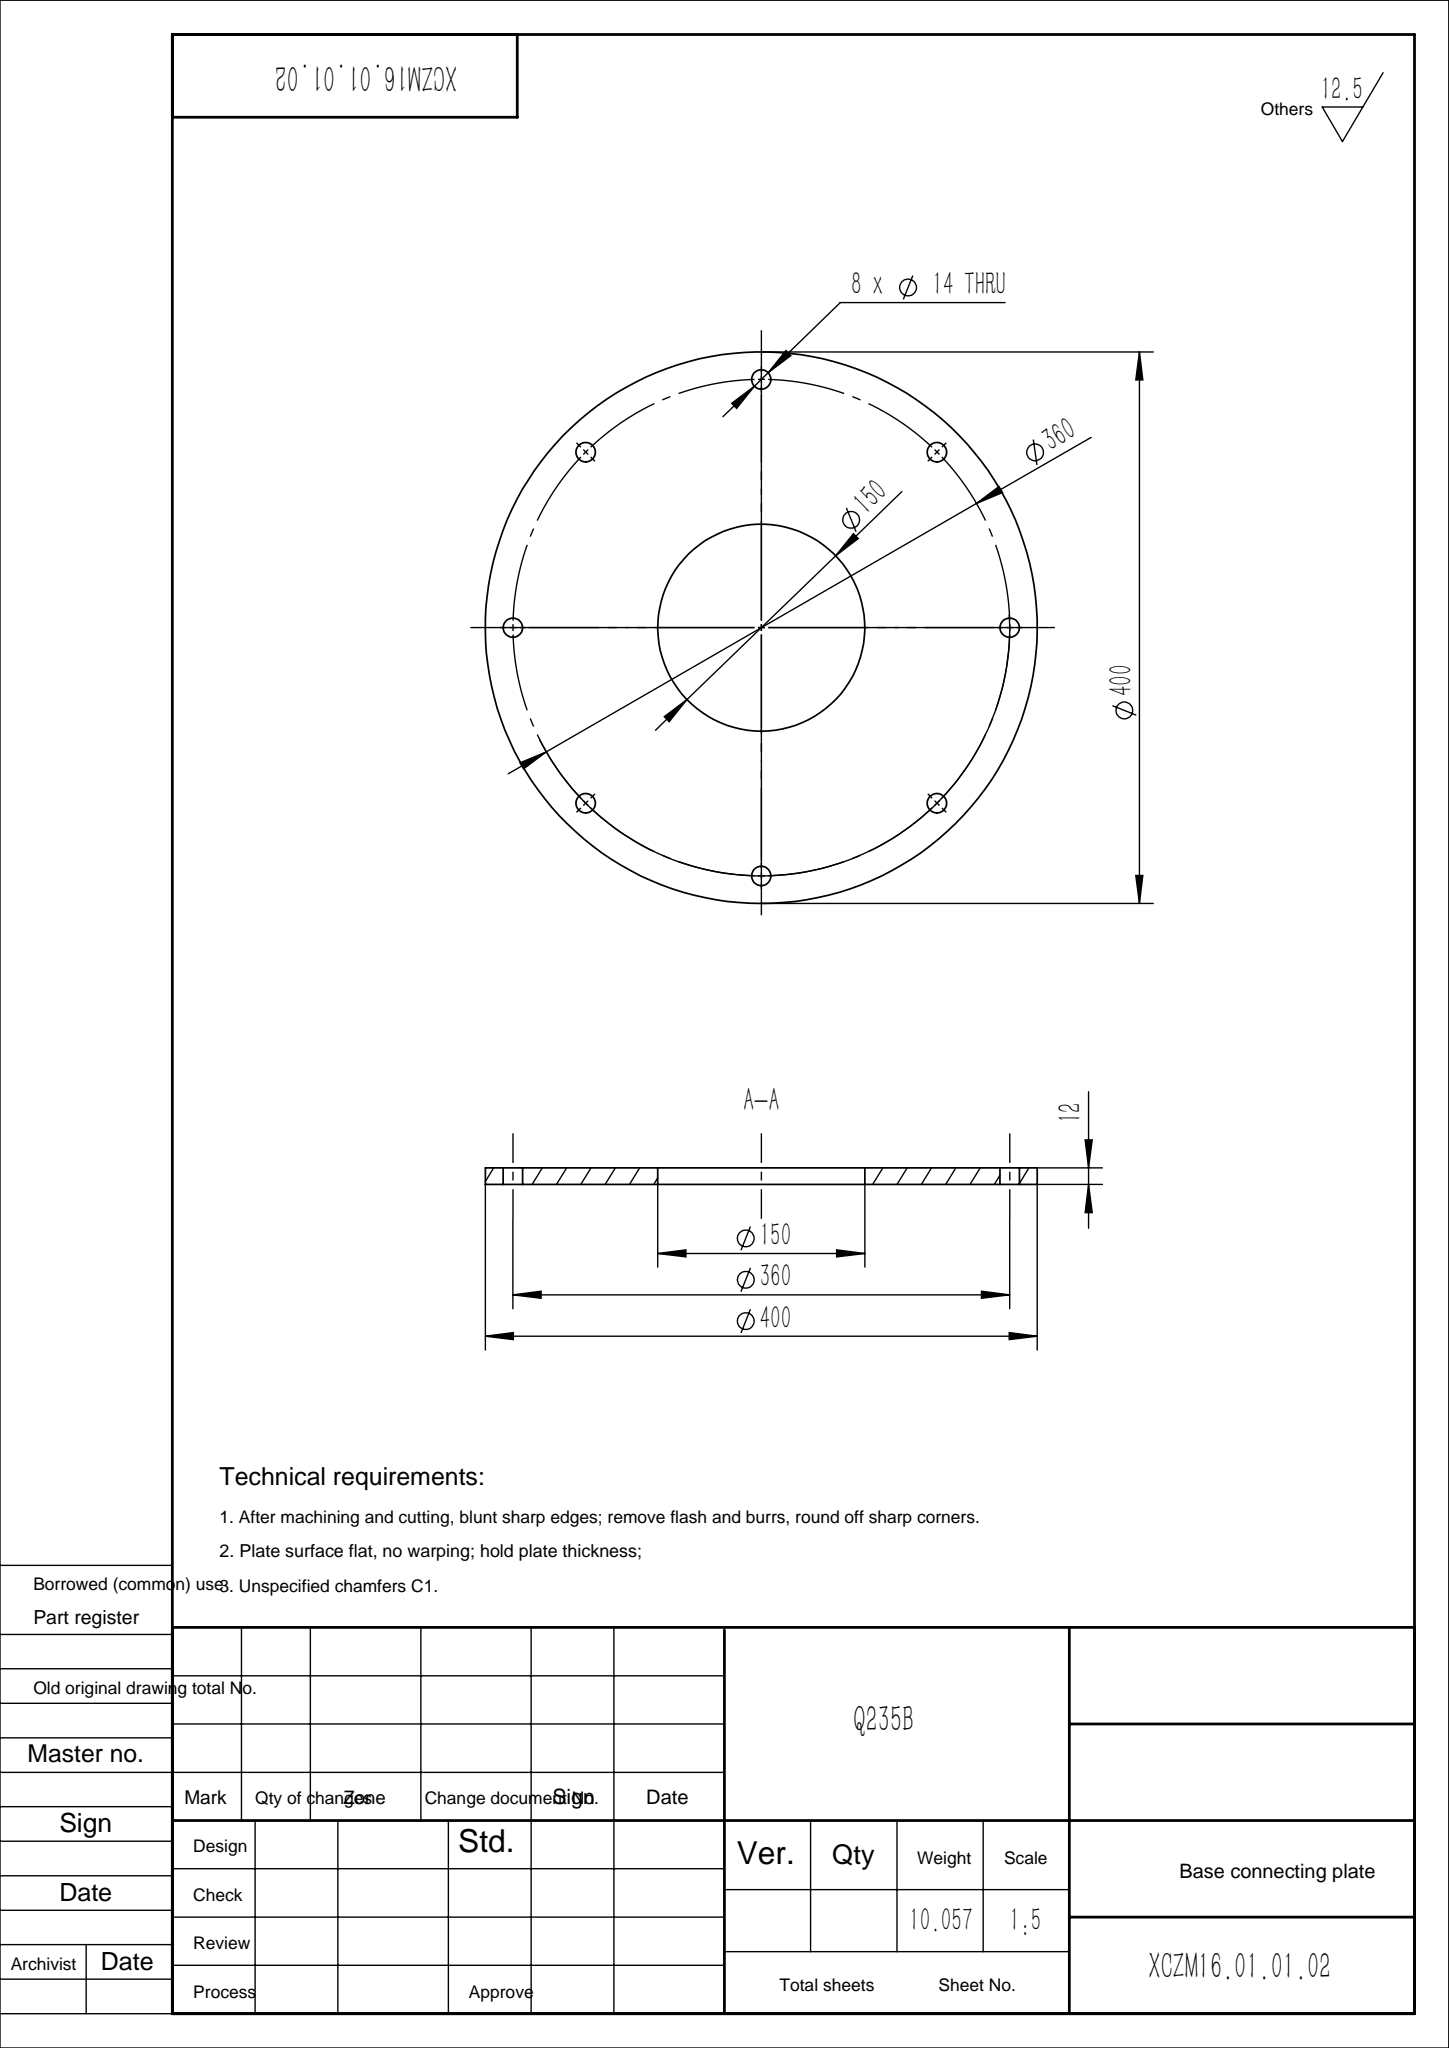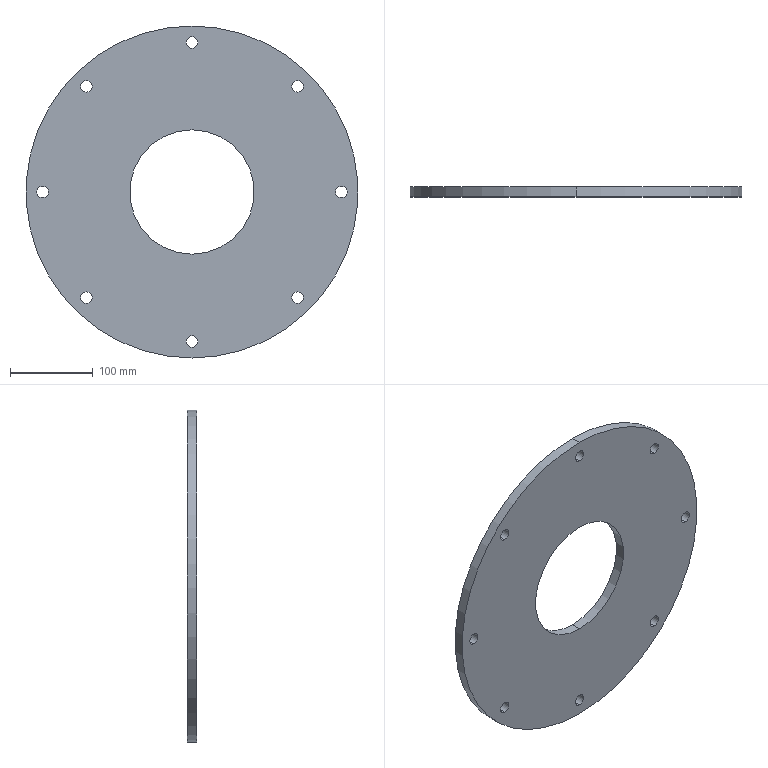Part | SolidWorks | features Extrusion 1, HoleWzd 1, RefAxis 1 | 1 solid | 22 faces | box 400 x 12 x 400 mm | volume 1281129 mm3 | cylinder 20 | plane 2 | commonest cylinder face diameters 14 x16 150 x2 400 x2
STEP:
#1=CARTESIAN_POINT('',(0.,0.,-187.));
#2=VERTEX_POINT('',#1);
#3=CARTESIAN_POINT('',(0.,0.,-173.));
#4=VERTEX_POINT('',#3);
#5=CARTESIAN_POINT('',(0.,0.,-180.));
#6=DIRECTION('',(0.,1.,0.));
#7=DIRECTION('',(0.,0.,1.));
#8=AXIS2_PLACEMENT_3D('',#5,#6,#7);
#9=CIRCLE('',#8,7.);
#10=EDGE_CURVE('',#2,#4,#9,.T.);
#11=ORIENTED_EDGE('',*,*,#10,.F.);
#12=CARTESIAN_POINT('',(0.,12.,-187.));
#13=VERTEX_POINT('',#12);
#14=CARTESIAN_POINT('',(0.,12.,-187.));
#15=DIRECTION('',(0.,1.,0.));
#16=VECTOR('',#15,1000.);
#17=LINE('',#14,#16);
#18=EDGE_CURVE('',#2,#13,#17,.T.);
#19=ORIENTED_EDGE('',*,*,#18,.T.);
#20=CARTESIAN_POINT('',(0.,12.,-173.));
#21=VERTEX_POINT('',#20);
#22=CARTESIAN_POINT('',(0.,12.,-180.));
#23=DIRECTION('',(0.,1.,0.));
#24=DIRECTION('',(0.,0.,1.));
#25=AXIS2_PLACEMENT_3D('',#22,#23,#24);
#26=CIRCLE('',#25,7.);
#27=EDGE_CURVE('',#13,#21,#26,.T.);
#28=ORIENTED_EDGE('',*,*,#27,.T.);
#29=CARTESIAN_POINT('',(0.,12.,-173.));
#30=DIRECTION('',(0.,1.,0.));
#31=VECTOR('',#30,1000.);
#32=LINE('',#29,#31);
#33=EDGE_CURVE('',#4,#21,#32,.T.);
#34=ORIENTED_EDGE('',*,*,#33,.F.);
#35=EDGE_LOOP('',(#11,#19,#28,#34));
#36=FACE_OUTER_BOUND('',#35,.T.);
#37=CARTESIAN_POINT('',(0.,12.,-180.));
#38=DIRECTION('',(0.,1.,0.));
#39=DIRECTION('',(0.,0.,1.));
#40=AXIS2_PLACEMENT_3D('',#37,#38,#39);
#41=CYLINDRICAL_SURFACE('',#40,7.);
#42=ADVANCED_FACE('',(#36),#41,.F.);
#43=CARTESIAN_POINT('',(127.279,0.,-134.279));
#44=VERTEX_POINT('',#43);
#45=CARTESIAN_POINT('',(127.279,0.,-120.279));
#46=VERTEX_POINT('',#45);
#47=CARTESIAN_POINT('',(127.279,0.,-127.279));
#48=DIRECTION('',(0.,1.,0.));
#49=DIRECTION('',(0.,0.,1.));
#50=AXIS2_PLACEMENT_3D('',#47,#48,#49);
#51=CIRCLE('',#50,7.);
#52=EDGE_CURVE('',#44,#46,#51,.T.);
#53=ORIENTED_EDGE('',*,*,#52,.F.);
#54=CARTESIAN_POINT('',(127.279,12.,-134.279));
#55=VERTEX_POINT('',#54);
#56=CARTESIAN_POINT('',(127.279,12.,-134.279));
#57=DIRECTION('',(0.,1.,0.));
#58=VECTOR('',#57,1000.);
#59=LINE('',#56,#58);
#60=EDGE_CURVE('',#44,#55,#59,.T.);
#61=ORIENTED_EDGE('',*,*,#60,.T.);
#62=CARTESIAN_POINT('',(127.279,12.,-120.279));
#63=VERTEX_POINT('',#62);
#64=CARTESIAN_POINT('',(127.279,12.,-127.279));
#65=DIRECTION('',(0.,1.,0.));
#66=DIRECTION('',(0.,0.,1.));
#67=AXIS2_PLACEMENT_3D('',#64,#65,#66);
#68=CIRCLE('',#67,7.);
#69=EDGE_CURVE('',#55,#63,#68,.T.);
#70=ORIENTED_EDGE('',*,*,#69,.T.);
#71=CARTESIAN_POINT('',(127.279,12.,-120.279));
#72=DIRECTION('',(0.,1.,0.));
#73=VECTOR('',#72,1000.);
#74=LINE('',#71,#73);
#75=EDGE_CURVE('',#46,#63,#74,.T.);
#76=ORIENTED_EDGE('',*,*,#75,.F.);
#77=EDGE_LOOP('',(#53,#61,#70,#76));
#78=FACE_OUTER_BOUND('',#77,.T.);
#79=CARTESIAN_POINT('',(127.279,12.,-127.279));
#80=DIRECTION('',(0.,1.,0.));
#81=DIRECTION('',(0.,0.,1.));
#82=AXIS2_PLACEMENT_3D('',#79,#80,#81);
#83=CYLINDRICAL_SURFACE('',#82,7.);
#84=ADVANCED_FACE('',(#78),#83,.F.);
#85=CARTESIAN_POINT('',(180.,0.,-7.));
#86=VERTEX_POINT('',#85);
#87=CARTESIAN_POINT('',(180.,0.,7.));
#88=VERTEX_POINT('',#87);
#89=CARTESIAN_POINT('',(180.,0.,0.));
#90=DIRECTION('',(0.,1.,0.));
#91=DIRECTION('',(0.,0.,1.));
#92=AXIS2_PLACEMENT_3D('',#89,#90,#91);
#93=CIRCLE('',#92,7.);
#94=EDGE_CURVE('',#86,#88,#93,.T.);
#95=ORIENTED_EDGE('',*,*,#94,.F.);
#96=CARTESIAN_POINT('',(180.,12.,-7.));
#97=VERTEX_POINT('',#96);
#98=CARTESIAN_POINT('',(180.,12.,-7.));
#99=DIRECTION('',(0.,1.,0.));
#100=VECTOR('',#99,1000.);
#101=LINE('',#98,#100);
#102=EDGE_CURVE('',#86,#97,#101,.T.);
#103=ORIENTED_EDGE('',*,*,#102,.T.);
#104=CARTESIAN_POINT('',(180.,12.,7.));
#105=VERTEX_POINT('',#104);
#106=CARTESIAN_POINT('',(180.,12.,0.));
#107=DIRECTION('',(0.,1.,0.));
#108=DIRECTION('',(0.,0.,1.));
#109=AXIS2_PLACEMENT_3D('',#106,#107,#108);
#110=CIRCLE('',#109,7.);
#111=EDGE_CURVE('',#97,#105,#110,.T.);
#112=ORIENTED_EDGE('',*,*,#111,.T.);
#113=CARTESIAN_POINT('',(180.,12.,7.));
#114=DIRECTION('',(0.,1.,0.));
#115=VECTOR('',#114,1000.);
#116=LINE('',#113,#115);
#117=EDGE_CURVE('',#88,#105,#116,.T.);
#118=ORIENTED_EDGE('',*,*,#117,.F.);
#119=EDGE_LOOP('',(#95,#103,#112,#118));
#120=FACE_OUTER_BOUND('',#119,.T.);
#121=CARTESIAN_POINT('',(180.,12.,0.));
#122=DIRECTION('',(0.,1.,0.));
#123=DIRECTION('',(0.,0.,1.));
#124=AXIS2_PLACEMENT_3D('',#121,#122,#123);
#125=CYLINDRICAL_SURFACE('',#124,7.);
#126=ADVANCED_FACE('',(#120),#125,.F.);
#127=CARTESIAN_POINT('',(127.279,0.,120.279));
#128=VERTEX_POINT('',#127);
#129=CARTESIAN_POINT('',(127.279,0.,134.279));
#130=VERTEX_POINT('',#129);
#131=CARTESIAN_POINT('',(127.279,0.,127.279));
#132=DIRECTION('',(0.,1.,0.));
#133=DIRECTION('',(0.,0.,1.));
#134=AXIS2_PLACEMENT_3D('',#131,#132,#133);
#135=CIRCLE('',#134,7.);
#136=EDGE_CURVE('',#128,#130,#135,.T.);
#137=ORIENTED_EDGE('',*,*,#136,.F.);
#138=CARTESIAN_POINT('',(127.279,12.,120.279));
#139=VERTEX_POINT('',#138);
#140=CARTESIAN_POINT('',(127.279,12.,120.279));
#141=DIRECTION('',(0.,1.,0.));
#142=VECTOR('',#141,1000.);
#143=LINE('',#140,#142);
#144=EDGE_CURVE('',#128,#139,#143,.T.);
#145=ORIENTED_EDGE('',*,*,#144,.T.);
#146=CARTESIAN_POINT('',(127.279,12.,134.279));
#147=VERTEX_POINT('',#146);
#148=CARTESIAN_POINT('',(127.279,12.,127.279));
#149=DIRECTION('',(0.,1.,0.));
#150=DIRECTION('',(0.,0.,1.));
#151=AXIS2_PLACEMENT_3D('',#148,#149,#150);
#152=CIRCLE('',#151,7.);
#153=EDGE_CURVE('',#139,#147,#152,.T.);
#154=ORIENTED_EDGE('',*,*,#153,.T.);
#155=CARTESIAN_POINT('',(127.279,12.,134.279));
#156=DIRECTION('',(0.,1.,0.));
#157=VECTOR('',#156,1000.);
#158=LINE('',#155,#157);
#159=EDGE_CURVE('',#130,#147,#158,.T.);
#160=ORIENTED_EDGE('',*,*,#159,.F.);
#161=EDGE_LOOP('',(#137,#145,#154,#160));
#162=FACE_OUTER_BOUND('',#161,.T.);
#163=CARTESIAN_POINT('',(127.279,12.,127.279));
#164=DIRECTION('',(0.,1.,0.));
#165=DIRECTION('',(0.,0.,1.));
#166=AXIS2_PLACEMENT_3D('',#163,#164,#165);
#167=CYLINDRICAL_SURFACE('',#166,7.);
#168=ADVANCED_FACE('',(#162),#167,.F.);
#169=CARTESIAN_POINT('',(0.,0.,173.));
#170=VERTEX_POINT('',#169);
#171=CARTESIAN_POINT('',(0.,0.,187.));
#172=VERTEX_POINT('',#171);
#173=CARTESIAN_POINT('',(0.,0.,180.));
#174=DIRECTION('',(0.,1.,0.));
#175=DIRECTION('',(0.,0.,1.));
#176=AXIS2_PLACEMENT_3D('',#173,#174,#175);
#177=CIRCLE('',#176,7.);
#178=EDGE_CURVE('',#170,#172,#177,.T.);
#179=ORIENTED_EDGE('',*,*,#178,.F.);
#180=CARTESIAN_POINT('',(0.,12.,173.));
#181=VERTEX_POINT('',#180);
#182=CARTESIAN_POINT('',(0.,12.,173.));
#183=DIRECTION('',(0.,1.,0.));
#184=VECTOR('',#183,1000.);
#185=LINE('',#182,#184);
#186=EDGE_CURVE('',#170,#181,#185,.T.);
#187=ORIENTED_EDGE('',*,*,#186,.T.);
#188=CARTESIAN_POINT('',(0.,12.,187.));
#189=VERTEX_POINT('',#188);
#190=CARTESIAN_POINT('',(0.,12.,180.));
#191=DIRECTION('',(0.,1.,0.));
#192=DIRECTION('',(0.,0.,1.));
#193=AXIS2_PLACEMENT_3D('',#190,#191,#192);
#194=CIRCLE('',#193,7.);
#195=EDGE_CURVE('',#181,#189,#194,.T.);
#196=ORIENTED_EDGE('',*,*,#195,.T.);
#197=CARTESIAN_POINT('',(0.,12.,187.));
#198=DIRECTION('',(0.,1.,0.));
#199=VECTOR('',#198,1000.);
#200=LINE('',#197,#199);
#201=EDGE_CURVE('',#172,#189,#200,.T.);
#202=ORIENTED_EDGE('',*,*,#201,.F.);
#203=EDGE_LOOP('',(#179,#187,#196,#202));
#204=FACE_OUTER_BOUND('',#203,.T.);
#205=CARTESIAN_POINT('',(0.,12.,180.));
#206=DIRECTION('',(0.,1.,0.));
#207=DIRECTION('',(0.,0.,1.));
#208=AXIS2_PLACEMENT_3D('',#205,#206,#207);
#209=CYLINDRICAL_SURFACE('',#208,7.);
#210=ADVANCED_FACE('',(#204),#209,.F.);
#211=CARTESIAN_POINT('',(-127.279,0.,120.279));
#212=VERTEX_POINT('',#211);
#213=CARTESIAN_POINT('',(-127.279,0.,134.279));
#214=VERTEX_POINT('',#213);
#215=CARTESIAN_POINT('',(-127.279,0.,127.279));
#216=DIRECTION('',(0.,1.,0.));
#217=DIRECTION('',(0.,0.,1.));
#218=AXIS2_PLACEMENT_3D('',#215,#216,#217);
#219=CIRCLE('',#218,7.);
#220=EDGE_CURVE('',#212,#214,#219,.T.);
#221=ORIENTED_EDGE('',*,*,#220,.F.);
#222=CARTESIAN_POINT('',(-127.279,12.,120.279));
#223=VERTEX_POINT('',#222);
#224=CARTESIAN_POINT('',(-127.279,12.,120.279));
#225=DIRECTION('',(0.,1.,0.));
#226=VECTOR('',#225,1000.);
#227=LINE('',#224,#226);
#228=EDGE_CURVE('',#212,#223,#227,.T.);
#229=ORIENTED_EDGE('',*,*,#228,.T.);
#230=CARTESIAN_POINT('',(-127.279,12.,134.279));
#231=VERTEX_POINT('',#230);
#232=CARTESIAN_POINT('',(-127.279,12.,127.279));
#233=DIRECTION('',(0.,1.,0.));
#234=DIRECTION('',(0.,0.,1.));
#235=AXIS2_PLACEMENT_3D('',#232,#233,#234);
#236=CIRCLE('',#235,7.);
#237=EDGE_CURVE('',#223,#231,#236,.T.);
#238=ORIENTED_EDGE('',*,*,#237,.T.);
#239=CARTESIAN_POINT('',(-127.279,12.,134.279));
#240=DIRECTION('',(0.,1.,0.));
#241=VECTOR('',#240,1000.);
#242=LINE('',#239,#241);
#243=EDGE_CURVE('',#214,#231,#242,.T.);
#244=ORIENTED_EDGE('',*,*,#243,.F.);
#245=EDGE_LOOP('',(#221,#229,#238,#244));
#246=FACE_OUTER_BOUND('',#245,.T.);
#247=CARTESIAN_POINT('',(-127.279,12.,127.279));
#248=DIRECTION('',(0.,1.,0.));
#249=DIRECTION('',(0.,0.,1.));
#250=AXIS2_PLACEMENT_3D('',#247,#248,#249);
#251=CYLINDRICAL_SURFACE('',#250,7.);
#252=ADVANCED_FACE('',(#246),#251,.F.);
#253=CARTESIAN_POINT('',(-180.,0.,-7.));
#254=VERTEX_POINT('',#253);
#255=CARTESIAN_POINT('',(-180.,0.,7.));
#256=VERTEX_POINT('',#255);
#257=CARTESIAN_POINT('',(-180.,0.,0.));
#258=DIRECTION('',(0.,1.,0.));
#259=DIRECTION('',(0.,0.,1.));
#260=AXIS2_PLACEMENT_3D('',#257,#258,#259);
#261=CIRCLE('',#260,7.);
#262=EDGE_CURVE('',#254,#256,#261,.T.);
#263=ORIENTED_EDGE('',*,*,#262,.F.);
#264=CARTESIAN_POINT('',(-180.,12.,-7.));
#265=VERTEX_POINT('',#264);
#266=CARTESIAN_POINT('',(-180.,12.,-7.));
#267=DIRECTION('',(0.,1.,0.));
#268=VECTOR('',#267,1000.);
#269=LINE('',#266,#268);
#270=EDGE_CURVE('',#254,#265,#269,.T.);
#271=ORIENTED_EDGE('',*,*,#270,.T.);
#272=CARTESIAN_POINT('',(-180.,12.,7.));
#273=VERTEX_POINT('',#272);
#274=CARTESIAN_POINT('',(-180.,12.,0.));
#275=DIRECTION('',(0.,1.,0.));
#276=DIRECTION('',(0.,0.,1.));
#277=AXIS2_PLACEMENT_3D('',#274,#275,#276);
#278=CIRCLE('',#277,7.);
#279=EDGE_CURVE('',#265,#273,#278,.T.);
#280=ORIENTED_EDGE('',*,*,#279,.T.);
#281=CARTESIAN_POINT('',(-180.,12.,7.));
#282=DIRECTION('',(0.,1.,0.));
#283=VECTOR('',#282,1000.);
#284=LINE('',#281,#283);
#285=EDGE_CURVE('',#256,#273,#284,.T.);
#286=ORIENTED_EDGE('',*,*,#285,.F.);
#287=EDGE_LOOP('',(#263,#271,#280,#286));
#288=FACE_OUTER_BOUND('',#287,.T.);
#289=CARTESIAN_POINT('',(-180.,12.,0.));
#290=DIRECTION('',(0.,1.,0.));
#291=DIRECTION('',(0.,0.,1.));
#292=AXIS2_PLACEMENT_3D('',#289,#290,#291);
#293=CYLINDRICAL_SURFACE('',#292,7.);
#294=ADVANCED_FACE('',(#288),#293,.F.);
#295=CARTESIAN_POINT('',(-127.279,0.,-134.279));
#296=VERTEX_POINT('',#295);
#297=CARTESIAN_POINT('',(-127.279,0.,-120.279));
#298=VERTEX_POINT('',#297);
#299=CARTESIAN_POINT('',(-127.279,0.,-127.279));
#300=DIRECTION('',(0.,1.,0.));
#301=DIRECTION('',(0.,0.,1.));
#302=AXIS2_PLACEMENT_3D('',#299,#300,#301);
#303=CIRCLE('',#302,7.);
#304=EDGE_CURVE('',#296,#298,#303,.T.);
#305=ORIENTED_EDGE('',*,*,#304,.F.);
#306=CARTESIAN_POINT('',(-127.279,12.,-134.279));
#307=VERTEX_POINT('',#306);
#308=CARTESIAN_POINT('',(-127.279,12.,-134.279));
#309=DIRECTION('',(0.,1.,0.));
#310=VECTOR('',#309,1000.);
#311=LINE('',#308,#310);
#312=EDGE_CURVE('',#296,#307,#311,.T.);
#313=ORIENTED_EDGE('',*,*,#312,.T.);
#314=CARTESIAN_POINT('',(-127.279,12.,-120.279));
#315=VERTEX_POINT('',#314);
#316=CARTESIAN_POINT('',(-127.279,12.,-127.279));
#317=DIRECTION('',(0.,1.,0.));
#318=DIRECTION('',(0.,0.,1.));
#319=AXIS2_PLACEMENT_3D('',#316,#317,#318);
#320=CIRCLE('',#319,7.);
#321=EDGE_CURVE('',#307,#315,#320,.T.);
#322=ORIENTED_EDGE('',*,*,#321,.T.);
#323=CARTESIAN_POINT('',(-127.279,12.,-120.279));
#324=DIRECTION('',(0.,1.,0.));
#325=VECTOR('',#324,1000.);
#326=LINE('',#323,#325);
#327=EDGE_CURVE('',#298,#315,#326,.T.);
#328=ORIENTED_EDGE('',*,*,#327,.F.);
#329=EDGE_LOOP('',(#305,#313,#322,#328));
#330=FACE_OUTER_BOUND('',#329,.T.);
#331=CARTESIAN_POINT('',(-127.279,12.,-127.279));
#332=DIRECTION('',(0.,1.,0.));
#333=DIRECTION('',(0.,0.,1.));
#334=AXIS2_PLACEMENT_3D('',#331,#332,#333);
#335=CYLINDRICAL_SURFACE('',#334,7.);
#336=ADVANCED_FACE('',(#330),#335,.F.);
#337=CARTESIAN_POINT('',(0.,12.,-75.));
#338=VERTEX_POINT('',#337);
#339=CARTESIAN_POINT('',(0.,12.,75.));
#340=VERTEX_POINT('',#339);
#341=CARTESIAN_POINT('',(0.,12.,0.));
#342=DIRECTION('',(0.,1.,0.));
#343=DIRECTION('',(0.,0.,1.));
#344=AXIS2_PLACEMENT_3D('',#341,#342,#343);
#345=CIRCLE('',#344,75.);
#346=EDGE_CURVE('',#338,#340,#345,.T.);
#347=ORIENTED_EDGE('',*,*,#346,.T.);
#348=CARTESIAN_POINT('',(0.,0.,75.));
#349=VERTEX_POINT('',#348);
#350=CARTESIAN_POINT('',(0.,12.,75.));
#351=DIRECTION('',(0.,-1.,0.));
#352=VECTOR('',#351,1000.);
#353=LINE('',#350,#352);
#354=EDGE_CURVE('',#340,#349,#353,.T.);
#355=ORIENTED_EDGE('',*,*,#354,.T.);
#356=CARTESIAN_POINT('',(0.,0.,-75.));
#357=VERTEX_POINT('',#356);
#358=CARTESIAN_POINT('',(0.,0.,0.));
#359=DIRECTION('',(0.,1.,0.));
#360=DIRECTION('',(0.,0.,1.));
#361=AXIS2_PLACEMENT_3D('',#358,#359,#360);
#362=CIRCLE('',#361,75.);
#363=EDGE_CURVE('',#357,#349,#362,.T.);
#364=ORIENTED_EDGE('',*,*,#363,.F.);
#365=CARTESIAN_POINT('',(0.,12.,-75.));
#366=DIRECTION('',(0.,-1.,0.));
#367=VECTOR('',#366,1000.);
#368=LINE('',#365,#367);
#369=EDGE_CURVE('',#338,#357,#368,.T.);
#370=ORIENTED_EDGE('',*,*,#369,.F.);
#371=EDGE_LOOP('',(#347,#355,#364,#370));
#372=FACE_OUTER_BOUND('',#371,.T.);
#373=CARTESIAN_POINT('',(0.,12.,0.));
#374=DIRECTION('',(0.,-1.,0.));
#375=DIRECTION('',(0.,0.,-1.));
#376=AXIS2_PLACEMENT_3D('',#373,#374,#375);
#377=CYLINDRICAL_SURFACE('',#376,75.);
#378=ADVANCED_FACE('',(#372),#377,.F.);
#379=CARTESIAN_POINT('',(0.,12.,200.));
#380=VERTEX_POINT('',#379);
#381=CARTESIAN_POINT('',(0.,12.,-200.));
#382=VERTEX_POINT('',#381);
#383=CARTESIAN_POINT('',(0.,12.,0.));
#384=DIRECTION('',(0.,1.,0.));
#385=DIRECTION('',(0.,0.,1.));
#386=AXIS2_PLACEMENT_3D('',#383,#384,#385);
#387=CIRCLE('',#386,200.);
#388=EDGE_CURVE('',#380,#382,#387,.T.);
#389=ORIENTED_EDGE('',*,*,#388,.F.);
#390=CARTESIAN_POINT('',(0.,0.,200.));
#391=VERTEX_POINT('',#390);
#392=CARTESIAN_POINT('',(0.,12.,200.));
#393=DIRECTION('',(0.,-1.,0.));
#394=VECTOR('',#393,1000.);
#395=LINE('',#392,#394);
#396=EDGE_CURVE('',#380,#391,#395,.T.);
#397=ORIENTED_EDGE('',*,*,#396,.T.);
#398=CARTESIAN_POINT('',(0.,0.,-200.));
#399=VERTEX_POINT('',#398);
#400=CARTESIAN_POINT('',(0.,0.,0.));
#401=DIRECTION('',(0.,1.,0.));
#402=DIRECTION('',(0.,0.,1.));
#403=AXIS2_PLACEMENT_3D('',#400,#401,#402);
#404=CIRCLE('',#403,200.);
#405=EDGE_CURVE('',#391,#399,#404,.T.);
#406=ORIENTED_EDGE('',*,*,#405,.T.);
#407=CARTESIAN_POINT('',(0.,12.,-200.));
#408=DIRECTION('',(0.,-1.,0.));
#409=VECTOR('',#408,1000.);
#410=LINE('',#407,#409);
#411=EDGE_CURVE('',#382,#399,#410,.T.);
#412=ORIENTED_EDGE('',*,*,#411,.F.);
#413=EDGE_LOOP('',(#389,#397,#406,#412));
#414=FACE_OUTER_BOUND('',#413,.T.);
#415=CARTESIAN_POINT('',(0.,12.,0.));
#416=DIRECTION('',(0.,-1.,0.));
#417=DIRECTION('',(0.,0.,-1.));
#418=AXIS2_PLACEMENT_3D('',#415,#416,#417);
#419=CYLINDRICAL_SURFACE('',#418,200.);
#420=ADVANCED_FACE('',(#414),#419,.T.);
#421=CARTESIAN_POINT('',(0.,12.,-180.));
#422=DIRECTION('',(0.,1.,0.));
#423=DIRECTION('',(0.,0.,1.));
#424=AXIS2_PLACEMENT_3D('',#421,#422,#423);
#425=CIRCLE('',#424,7.);
#426=EDGE_CURVE('',#21,#13,#425,.T.);
#427=ORIENTED_EDGE('',*,*,#426,.F.);
#428=ORIENTED_EDGE('',*,*,#27,.F.);
#429=EDGE_LOOP('',(#427,#428));
#430=FACE_BOUND('',#429,.T.);
#431=CARTESIAN_POINT('',(127.279,12.,-127.279));
#432=DIRECTION('',(0.,1.,0.));
#433=DIRECTION('',(0.,0.,1.));
#434=AXIS2_PLACEMENT_3D('',#431,#432,#433);
#435=CIRCLE('',#434,7.);
#436=EDGE_CURVE('',#63,#55,#435,.T.);
#437=ORIENTED_EDGE('',*,*,#436,.F.);
#438=ORIENTED_EDGE('',*,*,#69,.F.);
#439=EDGE_LOOP('',(#437,#438));
#440=FACE_BOUND('',#439,.T.);
#441=CARTESIAN_POINT('',(180.,12.,0.));
#442=DIRECTION('',(0.,1.,0.));
#443=DIRECTION('',(0.,0.,1.));
#444=AXIS2_PLACEMENT_3D('',#441,#442,#443);
#445=CIRCLE('',#444,7.);
#446=EDGE_CURVE('',#105,#97,#445,.T.);
#447=ORIENTED_EDGE('',*,*,#446,.F.);
#448=ORIENTED_EDGE('',*,*,#111,.F.);
#449=EDGE_LOOP('',(#447,#448));
#450=FACE_BOUND('',#449,.T.);
#451=CARTESIAN_POINT('',(127.279,12.,127.279));
#452=DIRECTION('',(0.,1.,0.));
#453=DIRECTION('',(0.,0.,1.));
#454=AXIS2_PLACEMENT_3D('',#451,#452,#453);
#455=CIRCLE('',#454,7.);
#456=EDGE_CURVE('',#147,#139,#455,.T.);
#457=ORIENTED_EDGE('',*,*,#456,.F.);
#458=ORIENTED_EDGE('',*,*,#153,.F.);
#459=EDGE_LOOP('',(#457,#458));
#460=FACE_BOUND('',#459,.T.);
#461=CARTESIAN_POINT('',(0.,12.,180.));
#462=DIRECTION('',(0.,1.,0.));
#463=DIRECTION('',(0.,0.,1.));
#464=AXIS2_PLACEMENT_3D('',#461,#462,#463);
#465=CIRCLE('',#464,7.);
#466=EDGE_CURVE('',#189,#181,#465,.T.);
#467=ORIENTED_EDGE('',*,*,#466,.F.);
#468=ORIENTED_EDGE('',*,*,#195,.F.);
#469=EDGE_LOOP('',(#467,#468));
#470=FACE_BOUND('',#469,.T.);
#471=CARTESIAN_POINT('',(-127.279,12.,127.279));
#472=DIRECTION('',(0.,1.,0.));
#473=DIRECTION('',(0.,0.,1.));
#474=AXIS2_PLACEMENT_3D('',#471,#472,#473);
#475=CIRCLE('',#474,7.);
#476=EDGE_CURVE('',#231,#223,#475,.T.);
#477=ORIENTED_EDGE('',*,*,#476,.F.);
#478=ORIENTED_EDGE('',*,*,#237,.F.);
#479=EDGE_LOOP('',(#477,#478));
#480=FACE_BOUND('',#479,.T.);
#481=CARTESIAN_POINT('',(-180.,12.,0.));
#482=DIRECTION('',(0.,1.,0.));
#483=DIRECTION('',(0.,0.,1.));
#484=AXIS2_PLACEMENT_3D('',#481,#482,#483);
#485=CIRCLE('',#484,7.);
#486=EDGE_CURVE('',#273,#265,#485,.T.);
#487=ORIENTED_EDGE('',*,*,#486,.F.);
#488=ORIENTED_EDGE('',*,*,#279,.F.);
#489=EDGE_LOOP('',(#487,#488));
#490=FACE_BOUND('',#489,.T.);
#491=CARTESIAN_POINT('',(-127.279,12.,-127.279));
#492=DIRECTION('',(0.,1.,0.));
#493=DIRECTION('',(0.,0.,1.));
#494=AXIS2_PLACEMENT_3D('',#491,#492,#493);
#495=CIRCLE('',#494,7.);
#496=EDGE_CURVE('',#315,#307,#495,.T.);
#497=ORIENTED_EDGE('',*,*,#496,.F.);
#498=ORIENTED_EDGE('',*,*,#321,.F.);
#499=EDGE_LOOP('',(#497,#498));
#500=FACE_BOUND('',#499,.T.);
#501=CARTESIAN_POINT('',(0.,12.,0.));
#502=DIRECTION('',(0.,1.,0.));
#503=DIRECTION('',(0.,0.,1.));
#504=AXIS2_PLACEMENT_3D('',#501,#502,#503);
#505=CIRCLE('',#504,200.);
#506=EDGE_CURVE('',#382,#380,#505,.T.);
#507=ORIENTED_EDGE('',*,*,#506,.T.);
#508=ORIENTED_EDGE('',*,*,#388,.T.);
#509=EDGE_LOOP('',(#507,#508));
#510=FACE_OUTER_BOUND('',#509,.T.);
#511=ORIENTED_EDGE('',*,*,#346,.F.);
#512=CARTESIAN_POINT('',(0.,12.,0.));
#513=DIRECTION('',(0.,1.,0.));
#514=DIRECTION('',(0.,0.,1.));
#515=AXIS2_PLACEMENT_3D('',#512,#513,#514);
#516=CIRCLE('',#515,75.);
#517=EDGE_CURVE('',#340,#338,#516,.T.);
#518=ORIENTED_EDGE('',*,*,#517,.F.);
#519=EDGE_LOOP('',(#511,#518));
#520=FACE_BOUND('',#519,.T.);
#521=CARTESIAN_POINT('',(0.,12.,0.));
#522=DIRECTION('',(0.,1.,0.));
#523=DIRECTION('',(0.,0.,1.));
#524=AXIS2_PLACEMENT_3D('',#521,#522,#523);
#525=PLANE('',#524);
#526=ADVANCED_FACE('',(#430,#440,#450,#460,#470,#480,#490,#500,#510,#520),#525,.T.);
#527=CARTESIAN_POINT('',(0.,0.,-180.));
#528=DIRECTION('',(0.,1.,0.));
#529=DIRECTION('',(0.,0.,1.));
#530=AXIS2_PLACEMENT_3D('',#527,#528,#529);
#531=CIRCLE('',#530,7.);
#532=EDGE_CURVE('',#4,#2,#531,.T.);
#533=ORIENTED_EDGE('',*,*,#532,.T.);
#534=ORIENTED_EDGE('',*,*,#10,.T.);
#535=EDGE_LOOP('',(#533,#534));
#536=FACE_BOUND('',#535,.T.);
#537=CARTESIAN_POINT('',(127.279,0.,-127.279));
#538=DIRECTION('',(0.,1.,0.));
#539=DIRECTION('',(0.,0.,1.));
#540=AXIS2_PLACEMENT_3D('',#537,#538,#539);
#541=CIRCLE('',#540,7.);
#542=EDGE_CURVE('',#46,#44,#541,.T.);
#543=ORIENTED_EDGE('',*,*,#542,.T.);
#544=ORIENTED_EDGE('',*,*,#52,.T.);
#545=EDGE_LOOP('',(#543,#544));
#546=FACE_BOUND('',#545,.T.);
#547=CARTESIAN_POINT('',(180.,0.,0.));
#548=DIRECTION('',(0.,1.,0.));
#549=DIRECTION('',(0.,0.,1.));
#550=AXIS2_PLACEMENT_3D('',#547,#548,#549);
#551=CIRCLE('',#550,7.);
#552=EDGE_CURVE('',#88,#86,#551,.T.);
#553=ORIENTED_EDGE('',*,*,#552,.T.);
#554=ORIENTED_EDGE('',*,*,#94,.T.);
#555=EDGE_LOOP('',(#553,#554));
#556=FACE_BOUND('',#555,.T.);
#557=CARTESIAN_POINT('',(127.279,0.,127.279));
#558=DIRECTION('',(0.,1.,0.));
#559=DIRECTION('',(0.,0.,1.));
#560=AXIS2_PLACEMENT_3D('',#557,#558,#559);
#561=CIRCLE('',#560,7.);
#562=EDGE_CURVE('',#130,#128,#561,.T.);
#563=ORIENTED_EDGE('',*,*,#562,.T.);
#564=ORIENTED_EDGE('',*,*,#136,.T.);
#565=EDGE_LOOP('',(#563,#564));
#566=FACE_BOUND('',#565,.T.);
#567=CARTESIAN_POINT('',(0.,0.,180.));
#568=DIRECTION('',(0.,1.,0.));
#569=DIRECTION('',(0.,0.,1.));
#570=AXIS2_PLACEMENT_3D('',#567,#568,#569);
#571=CIRCLE('',#570,7.);
#572=EDGE_CURVE('',#172,#170,#571,.T.);
#573=ORIENTED_EDGE('',*,*,#572,.T.);
#574=ORIENTED_EDGE('',*,*,#178,.T.);
#575=EDGE_LOOP('',(#573,#574));
#576=FACE_BOUND('',#575,.T.);
#577=CARTESIAN_POINT('',(-127.279,0.,127.279));
#578=DIRECTION('',(0.,1.,0.));
#579=DIRECTION('',(0.,0.,1.));
#580=AXIS2_PLACEMENT_3D('',#577,#578,#579);
#581=CIRCLE('',#580,7.);
#582=EDGE_CURVE('',#214,#212,#581,.T.);
#583=ORIENTED_EDGE('',*,*,#582,.T.);
#584=ORIENTED_EDGE('',*,*,#220,.T.);
#585=EDGE_LOOP('',(#583,#584));
#586=FACE_BOUND('',#585,.T.);
#587=CARTESIAN_POINT('',(-180.,0.,0.));
#588=DIRECTION('',(0.,1.,0.));
#589=DIRECTION('',(0.,0.,1.));
#590=AXIS2_PLACEMENT_3D('',#587,#588,#589);
#591=CIRCLE('',#590,7.);
#592=EDGE_CURVE('',#256,#254,#591,.T.);
#593=ORIENTED_EDGE('',*,*,#592,.T.);
#594=ORIENTED_EDGE('',*,*,#262,.T.);
#595=EDGE_LOOP('',(#593,#594));
#596=FACE_BOUND('',#595,.T.);
#597=CARTESIAN_POINT('',(-127.279,0.,-127.279));
#598=DIRECTION('',(0.,1.,0.));
#599=DIRECTION('',(0.,0.,1.));
#600=AXIS2_PLACEMENT_3D('',#597,#598,#599);
#601=CIRCLE('',#600,7.);
#602=EDGE_CURVE('',#298,#296,#601,.T.);
#603=ORIENTED_EDGE('',*,*,#602,.T.);
#604=ORIENTED_EDGE('',*,*,#304,.T.);
#605=EDGE_LOOP('',(#603,#604));
#606=FACE_BOUND('',#605,.T.);
#607=CARTESIAN_POINT('',(0.,0.,0.));
#608=DIRECTION('',(0.,1.,0.));
#609=DIRECTION('',(0.,0.,1.));
#610=AXIS2_PLACEMENT_3D('',#607,#608,#609);
#611=CIRCLE('',#610,200.);
#612=EDGE_CURVE('',#399,#391,#611,.T.);
#613=ORIENTED_EDGE('',*,*,#612,.F.);
#614=ORIENTED_EDGE('',*,*,#405,.F.);
#615=EDGE_LOOP('',(#613,#614));
#616=FACE_OUTER_BOUND('',#615,.T.);
#617=ORIENTED_EDGE('',*,*,#363,.T.);
#618=CARTESIAN_POINT('',(0.,0.,0.));
#619=DIRECTION('',(0.,1.,0.));
#620=DIRECTION('',(0.,0.,1.));
#621=AXIS2_PLACEMENT_3D('',#618,#619,#620);
#622=CIRCLE('',#621,75.);
#623=EDGE_CURVE('',#349,#357,#622,.T.);
#624=ORIENTED_EDGE('',*,*,#623,.T.);
#625=EDGE_LOOP('',(#617,#624));
#626=FACE_BOUND('',#625,.T.);
#627=CARTESIAN_POINT('',(0.,0.,0.));
#628=DIRECTION('',(0.,1.,0.));
#629=DIRECTION('',(0.,0.,1.));
#630=AXIS2_PLACEMENT_3D('',#627,#628,#629);
#631=PLANE('',#630);
#632=ADVANCED_FACE('',(#536,#546,#556,#566,#576,#586,#596,#606,#616,#626),#631,.F.);
#633=ORIENTED_EDGE('',*,*,#396,.F.);
#634=ORIENTED_EDGE('',*,*,#506,.F.);
#635=ORIENTED_EDGE('',*,*,#411,.T.);
#636=ORIENTED_EDGE('',*,*,#612,.T.);
#637=EDGE_LOOP('',(#633,#634,#635,#636));
#638=FACE_OUTER_BOUND('',#637,.T.);
#639=CARTESIAN_POINT('',(0.,12.,0.));
#640=DIRECTION('',(0.,-1.,0.));
#641=DIRECTION('',(0.,0.,-1.));
#642=AXIS2_PLACEMENT_3D('',#639,#640,#641);
#643=CYLINDRICAL_SURFACE('',#642,200.);
#644=ADVANCED_FACE('',(#638),#643,.T.);
#645=ORIENTED_EDGE('',*,*,#354,.F.);
#646=ORIENTED_EDGE('',*,*,#517,.T.);
#647=ORIENTED_EDGE('',*,*,#369,.T.);
#648=ORIENTED_EDGE('',*,*,#623,.F.);
#649=EDGE_LOOP('',(#645,#646,#647,#648));
#650=FACE_OUTER_BOUND('',#649,.T.);
#651=CARTESIAN_POINT('',(0.,12.,0.));
#652=DIRECTION('',(0.,-1.,0.));
#653=DIRECTION('',(0.,0.,-1.));
#654=AXIS2_PLACEMENT_3D('',#651,#652,#653);
#655=CYLINDRICAL_SURFACE('',#654,75.);
#656=ADVANCED_FACE('',(#650),#655,.F.);
#657=ORIENTED_EDGE('',*,*,#312,.F.);
#658=ORIENTED_EDGE('',*,*,#602,.F.);
#659=ORIENTED_EDGE('',*,*,#327,.T.);
#660=ORIENTED_EDGE('',*,*,#496,.T.);
#661=EDGE_LOOP('',(#657,#658,#659,#660));
#662=FACE_OUTER_BOUND('',#661,.T.);
#663=CARTESIAN_POINT('',(-127.279,12.,-127.279));
#664=DIRECTION('',(0.,1.,0.));
#665=DIRECTION('',(0.,0.,1.));
#666=AXIS2_PLACEMENT_3D('',#663,#664,#665);
#667=CYLINDRICAL_SURFACE('',#666,7.);
#668=ADVANCED_FACE('',(#662),#667,.F.);
#669=ORIENTED_EDGE('',*,*,#270,.F.);
#670=ORIENTED_EDGE('',*,*,#592,.F.);
#671=ORIENTED_EDGE('',*,*,#285,.T.);
#672=ORIENTED_EDGE('',*,*,#486,.T.);
#673=EDGE_LOOP('',(#669,#670,#671,#672));
#674=FACE_OUTER_BOUND('',#673,.T.);
#675=CARTESIAN_POINT('',(-180.,12.,0.));
#676=DIRECTION('',(0.,1.,0.));
#677=DIRECTION('',(0.,0.,1.));
#678=AXIS2_PLACEMENT_3D('',#675,#676,#677);
#679=CYLINDRICAL_SURFACE('',#678,7.);
#680=ADVANCED_FACE('',(#674),#679,.F.);
#681=ORIENTED_EDGE('',*,*,#228,.F.);
#682=ORIENTED_EDGE('',*,*,#582,.F.);
#683=ORIENTED_EDGE('',*,*,#243,.T.);
#684=ORIENTED_EDGE('',*,*,#476,.T.);
#685=EDGE_LOOP('',(#681,#682,#683,#684));
#686=FACE_OUTER_BOUND('',#685,.T.);
#687=CARTESIAN_POINT('',(-127.279,12.,127.279));
#688=DIRECTION('',(0.,1.,0.));
#689=DIRECTION('',(0.,0.,1.));
#690=AXIS2_PLACEMENT_3D('',#687,#688,#689);
#691=CYLINDRICAL_SURFACE('',#690,7.);
#692=ADVANCED_FACE('',(#686),#691,.F.);
#693=ORIENTED_EDGE('',*,*,#186,.F.);
#694=ORIENTED_EDGE('',*,*,#572,.F.);
#695=ORIENTED_EDGE('',*,*,#201,.T.);
#696=ORIENTED_EDGE('',*,*,#466,.T.);
#697=EDGE_LOOP('',(#693,#694,#695,#696));
#698=FACE_OUTER_BOUND('',#697,.T.);
#699=CARTESIAN_POINT('',(0.,12.,180.));
#700=DIRECTION('',(0.,1.,0.));
#701=DIRECTION('',(0.,0.,1.));
#702=AXIS2_PLACEMENT_3D('',#699,#700,#701);
#703=CYLINDRICAL_SURFACE('',#702,7.);
#704=ADVANCED_FACE('',(#698),#703,.F.);
#705=ORIENTED_EDGE('',*,*,#144,.F.);
#706=ORIENTED_EDGE('',*,*,#562,.F.);
#707=ORIENTED_EDGE('',*,*,#159,.T.);
#708=ORIENTED_EDGE('',*,*,#456,.T.);
#709=EDGE_LOOP('',(#705,#706,#707,#708));
#710=FACE_OUTER_BOUND('',#709,.T.);
#711=CARTESIAN_POINT('',(127.279,12.,127.279));
#712=DIRECTION('',(0.,1.,0.));
#713=DIRECTION('',(0.,0.,1.));
#714=AXIS2_PLACEMENT_3D('',#711,#712,#713);
#715=CYLINDRICAL_SURFACE('',#714,7.);
#716=ADVANCED_FACE('',(#710),#715,.F.);
#717=ORIENTED_EDGE('',*,*,#102,.F.);
#718=ORIENTED_EDGE('',*,*,#552,.F.);
#719=ORIENTED_EDGE('',*,*,#117,.T.);
#720=ORIENTED_EDGE('',*,*,#446,.T.);
#721=EDGE_LOOP('',(#717,#718,#719,#720));
#722=FACE_OUTER_BOUND('',#721,.T.);
#723=CARTESIAN_POINT('',(180.,12.,0.));
#724=DIRECTION('',(0.,1.,0.));
#725=DIRECTION('',(0.,0.,1.));
#726=AXIS2_PLACEMENT_3D('',#723,#724,#725);
#727=CYLINDRICAL_SURFACE('',#726,7.);
#728=ADVANCED_FACE('',(#722),#727,.F.);
#729=ORIENTED_EDGE('',*,*,#60,.F.);
#730=ORIENTED_EDGE('',*,*,#542,.F.);
#731=ORIENTED_EDGE('',*,*,#75,.T.);
#732=ORIENTED_EDGE('',*,*,#436,.T.);
#733=EDGE_LOOP('',(#729,#730,#731,#732));
#734=FACE_OUTER_BOUND('',#733,.T.);
#735=CARTESIAN_POINT('',(127.279,12.,-127.279));
#736=DIRECTION('',(0.,1.,0.));
#737=DIRECTION('',(0.,0.,1.));
#738=AXIS2_PLACEMENT_3D('',#735,#736,#737);
#739=CYLINDRICAL_SURFACE('',#738,7.);
#740=ADVANCED_FACE('',(#734),#739,.F.);
#741=ORIENTED_EDGE('',*,*,#18,.F.);
#742=ORIENTED_EDGE('',*,*,#532,.F.);
#743=ORIENTED_EDGE('',*,*,#33,.T.);
#744=ORIENTED_EDGE('',*,*,#426,.T.);
#745=EDGE_LOOP('',(#741,#742,#743,#744));
#746=FACE_OUTER_BOUND('',#745,.T.);
#747=CARTESIAN_POINT('',(0.,12.,-180.));
#748=DIRECTION('',(0.,1.,0.));
#749=DIRECTION('',(0.,0.,1.));
#750=AXIS2_PLACEMENT_3D('',#747,#748,#749);
#751=CYLINDRICAL_SURFACE('',#750,7.);
#752=ADVANCED_FACE('',(#746),#751,.F.);
#753=CLOSED_SHELL('',(#42,#84,#126,#168,#210,#252,#294,#336,#378,#420,#526,#632,#644,#656,#668,#680,#692,#704,#716,#728,#740,#752));
#754=MANIFOLD_SOLID_BREP('',#753);
#755=CARTESIAN_POINT('',(0.,0.,0.));
#756=DIRECTION('',(0.,0.,1.));
#757=DIRECTION('',(1.,0.,0.));
#758=AXIS2_PLACEMENT_3D('',#755,#756,#757);
#759=(LENGTH_UNIT()NAMED_UNIT(*)SI_UNIT(.MILLI.,.METRE.));
#760=UNCERTAINTY_MEASURE_WITH_UNIT(LENGTH_MEASURE(0.00001),#759,'','');
#761=(NAMED_UNIT(*)PLANE_ANGLE_UNIT()SI_UNIT($,.RADIAN.));
#762=(NAMED_UNIT(*)SI_UNIT($,.STERADIAN.)SOLID_ANGLE_UNIT());
#763=(GEOMETRIC_REPRESENTATION_CONTEXT(3)GLOBAL_UNCERTAINTY_ASSIGNED_CONTEXT((#760))GLOBAL_UNIT_ASSIGNED_CONTEXT((#759,#761,#762))REPRESENTATION_CONTEXT('',''));
#764=ADVANCED_BREP_SHAPE_REPRESENTATION('',(#754,#758),#763);